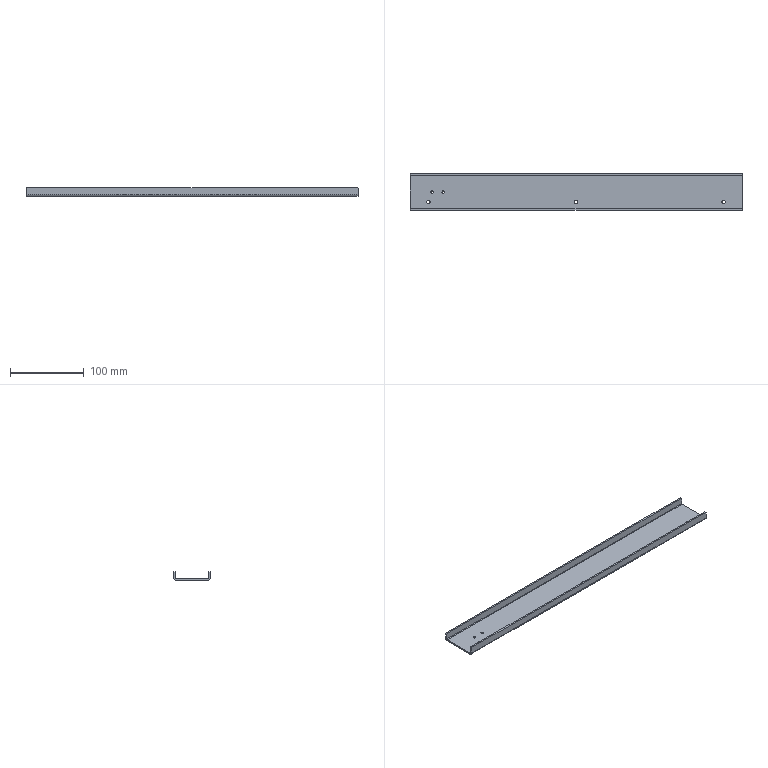Part | NX | features BREP 1 | 1 solid | 36 faces | box 450 x 49 x 12 mm | volume 60625 mm3 | plane 22 | cylinder 14 | commonest cylinder face diameters 4.5 x6 3.3 x4 1.473 x2 5.473 x2
STEP:
#1=CARTESIAN_POINT('',(27.25,9.,-2.));
#2=VERTEX_POINT('',#1);
#3=CARTESIAN_POINT('',(22.75,9.,-2.));
#4=VERTEX_POINT('',#3);
#5=CARTESIAN_POINT('',(25.,9.,-2.));
#6=DIRECTION('',(0.,0.,-1.));
#7=DIRECTION('',(-1.,0.,0.));
#8=AXIS2_PLACEMENT_3D('',#5,#6,#7);
#9=CIRCLE('',#8,2.25);
#10=EDGE_CURVE('',#2,#4,#9,.T.);
#11=ORIENTED_EDGE('',*,*,#10,.T.);
#12=CARTESIAN_POINT('',(22.75,9.,0.));
#13=VERTEX_POINT('',#12);
#14=CARTESIAN_POINT('',(22.75,9.,0.));
#15=DIRECTION('',(0.,0.,1.));
#16=VECTOR('',#15,1000.);
#17=LINE('',#14,#16);
#18=EDGE_CURVE('',#13,#4,#17,.F.);
#19=ORIENTED_EDGE('',*,*,#18,.F.);
#20=CARTESIAN_POINT('',(27.25,9.,0.));
#21=VERTEX_POINT('',#20);
#22=CARTESIAN_POINT('',(25.,9.,0.));
#23=DIRECTION('',(0.,0.,1.));
#24=DIRECTION('',(1.,0.,0.));
#25=AXIS2_PLACEMENT_3D('',#22,#23,#24);
#26=CIRCLE('',#25,2.25);
#27=EDGE_CURVE('',#13,#21,#26,.T.);
#28=ORIENTED_EDGE('',*,*,#27,.T.);
#29=CARTESIAN_POINT('',(27.25,9.,0.));
#30=DIRECTION('',(0.,0.,1.));
#31=VECTOR('',#30,1000.);
#32=LINE('',#29,#31);
#33=EDGE_CURVE('',#21,#2,#32,.F.);
#34=ORIENTED_EDGE('',*,*,#33,.T.);
#35=EDGE_LOOP('',(#11,#19,#28,#34));
#36=FACE_BOUND('',#35,.T.);
#37=CARTESIAN_POINT('',(25.,9.,0.));
#38=DIRECTION('',(0.,0.,1.));
#39=DIRECTION('',(1.,0.,0.));
#40=AXIS2_PLACEMENT_3D('',#37,#38,#39);
#41=CYLINDRICAL_SURFACE('',#40,2.25);
#42=ADVANCED_FACE('',(#36),#41,.F.);
#43=CARTESIAN_POINT('',(227.25,9.,-2.));
#44=VERTEX_POINT('',#43);
#45=CARTESIAN_POINT('',(222.75,9.,-2.));
#46=VERTEX_POINT('',#45);
#47=CARTESIAN_POINT('',(225.,9.,-2.));
#48=DIRECTION('',(0.,0.,-1.));
#49=DIRECTION('',(-1.,0.,0.));
#50=AXIS2_PLACEMENT_3D('',#47,#48,#49);
#51=CIRCLE('',#50,2.25);
#52=EDGE_CURVE('',#44,#46,#51,.T.);
#53=ORIENTED_EDGE('',*,*,#52,.T.);
#54=CARTESIAN_POINT('',(222.75,9.,0.));
#55=VERTEX_POINT('',#54);
#56=CARTESIAN_POINT('',(222.75,9.,0.));
#57=DIRECTION('',(0.,0.,1.));
#58=VECTOR('',#57,1000.);
#59=LINE('',#56,#58);
#60=EDGE_CURVE('',#55,#46,#59,.F.);
#61=ORIENTED_EDGE('',*,*,#60,.F.);
#62=CARTESIAN_POINT('',(227.25,9.,0.));
#63=VERTEX_POINT('',#62);
#64=CARTESIAN_POINT('',(225.,9.,0.));
#65=DIRECTION('',(0.,0.,1.));
#66=DIRECTION('',(1.,0.,0.));
#67=AXIS2_PLACEMENT_3D('',#64,#65,#66);
#68=CIRCLE('',#67,2.25);
#69=EDGE_CURVE('',#55,#63,#68,.T.);
#70=ORIENTED_EDGE('',*,*,#69,.T.);
#71=CARTESIAN_POINT('',(227.25,9.,0.));
#72=DIRECTION('',(0.,0.,1.));
#73=VECTOR('',#72,1000.);
#74=LINE('',#71,#73);
#75=EDGE_CURVE('',#63,#44,#74,.F.);
#76=ORIENTED_EDGE('',*,*,#75,.T.);
#77=EDGE_LOOP('',(#53,#61,#70,#76));
#78=FACE_BOUND('',#77,.T.);
#79=CARTESIAN_POINT('',(225.,9.,0.));
#80=DIRECTION('',(0.,0.,1.));
#81=DIRECTION('',(1.,0.,0.));
#82=AXIS2_PLACEMENT_3D('',#79,#80,#81);
#83=CYLINDRICAL_SURFACE('',#82,2.25);
#84=ADVANCED_FACE('',(#78),#83,.F.);
#85=CARTESIAN_POINT('',(427.25,9.,-2.));
#86=VERTEX_POINT('',#85);
#87=CARTESIAN_POINT('',(422.75,9.,-2.));
#88=VERTEX_POINT('',#87);
#89=CARTESIAN_POINT('',(425.,9.,-2.));
#90=DIRECTION('',(0.,0.,-1.));
#91=DIRECTION('',(-1.,0.,0.));
#92=AXIS2_PLACEMENT_3D('',#89,#90,#91);
#93=CIRCLE('',#92,2.25);
#94=EDGE_CURVE('',#86,#88,#93,.T.);
#95=ORIENTED_EDGE('',*,*,#94,.T.);
#96=CARTESIAN_POINT('',(422.75,9.,0.));
#97=VERTEX_POINT('',#96);
#98=CARTESIAN_POINT('',(422.75,9.,0.));
#99=DIRECTION('',(0.,0.,1.));
#100=VECTOR('',#99,1000.);
#101=LINE('',#98,#100);
#102=EDGE_CURVE('',#97,#88,#101,.F.);
#103=ORIENTED_EDGE('',*,*,#102,.F.);
#104=CARTESIAN_POINT('',(427.25,9.,0.));
#105=VERTEX_POINT('',#104);
#106=CARTESIAN_POINT('',(425.,9.,0.));
#107=DIRECTION('',(0.,0.,1.));
#108=DIRECTION('',(1.,0.,0.));
#109=AXIS2_PLACEMENT_3D('',#106,#107,#108);
#110=CIRCLE('',#109,2.25);
#111=EDGE_CURVE('',#97,#105,#110,.T.);
#112=ORIENTED_EDGE('',*,*,#111,.T.);
#113=CARTESIAN_POINT('',(427.25,9.,0.));
#114=DIRECTION('',(0.,0.,1.));
#115=VECTOR('',#114,1000.);
#116=LINE('',#113,#115);
#117=EDGE_CURVE('',#105,#86,#116,.F.);
#118=ORIENTED_EDGE('',*,*,#117,.T.);
#119=EDGE_LOOP('',(#95,#103,#112,#118));
#120=FACE_BOUND('',#119,.T.);
#121=CARTESIAN_POINT('',(425.,9.,0.));
#122=DIRECTION('',(0.,0.,1.));
#123=DIRECTION('',(1.,0.,0.));
#124=AXIS2_PLACEMENT_3D('',#121,#122,#123);
#125=CYLINDRICAL_SURFACE('',#124,2.25);
#126=ADVANCED_FACE('',(#120),#125,.F.);
#127=CARTESIAN_POINT('',(28.35,22.5,-2.));
#128=VERTEX_POINT('',#127);
#129=CARTESIAN_POINT('',(31.65,22.5,-2.));
#130=VERTEX_POINT('',#129);
#131=CARTESIAN_POINT('',(30.,22.5,-2.));
#132=DIRECTION('',(0.,0.,1.));
#133=DIRECTION('',(1.,0.,0.));
#134=AXIS2_PLACEMENT_3D('',#131,#132,#133);
#135=CIRCLE('',#134,1.65);
#136=EDGE_CURVE('',#128,#130,#135,.T.);
#137=ORIENTED_EDGE('',*,*,#136,.F.);
#138=CARTESIAN_POINT('',(28.35,22.5,0.));
#139=VERTEX_POINT('',#138);
#140=CARTESIAN_POINT('',(28.35,22.5,0.));
#141=DIRECTION('',(0.,0.,1.));
#142=VECTOR('',#141,1000.);
#143=LINE('',#140,#142);
#144=EDGE_CURVE('',#139,#128,#143,.F.);
#145=ORIENTED_EDGE('',*,*,#144,.F.);
#146=CARTESIAN_POINT('',(31.65,22.5,0.));
#147=VERTEX_POINT('',#146);
#148=CARTESIAN_POINT('',(30.,22.5,0.));
#149=DIRECTION('',(0.,0.,1.));
#150=DIRECTION('',(1.,0.,0.));
#151=AXIS2_PLACEMENT_3D('',#148,#149,#150);
#152=CIRCLE('',#151,1.65);
#153=EDGE_CURVE('',#139,#147,#152,.T.);
#154=ORIENTED_EDGE('',*,*,#153,.T.);
#155=CARTESIAN_POINT('',(31.65,22.5,0.));
#156=DIRECTION('',(0.,0.,1.));
#157=VECTOR('',#156,1000.);
#158=LINE('',#155,#157);
#159=EDGE_CURVE('',#147,#130,#158,.F.);
#160=ORIENTED_EDGE('',*,*,#159,.T.);
#161=EDGE_LOOP('',(#137,#145,#154,#160));
#162=FACE_BOUND('',#161,.T.);
#163=CARTESIAN_POINT('',(30.,22.5,0.));
#164=DIRECTION('',(0.,0.,1.));
#165=DIRECTION('',(1.,0.,0.));
#166=AXIS2_PLACEMENT_3D('',#163,#164,#165);
#167=CYLINDRICAL_SURFACE('',#166,1.65);
#168=ADVANCED_FACE('',(#162),#167,.F.);
#169=CARTESIAN_POINT('',(43.35,22.5,-2.));
#170=VERTEX_POINT('',#169);
#171=CARTESIAN_POINT('',(46.65,22.5,-2.));
#172=VERTEX_POINT('',#171);
#173=CARTESIAN_POINT('',(45.,22.5,-2.));
#174=DIRECTION('',(0.,0.,1.));
#175=DIRECTION('',(1.,0.,0.));
#176=AXIS2_PLACEMENT_3D('',#173,#174,#175);
#177=CIRCLE('',#176,1.65);
#178=EDGE_CURVE('',#170,#172,#177,.T.);
#179=ORIENTED_EDGE('',*,*,#178,.F.);
#180=CARTESIAN_POINT('',(43.35,22.5,0.));
#181=VERTEX_POINT('',#180);
#182=CARTESIAN_POINT('',(43.35,22.5,0.));
#183=DIRECTION('',(0.,0.,1.));
#184=VECTOR('',#183,1000.);
#185=LINE('',#182,#184);
#186=EDGE_CURVE('',#181,#170,#185,.F.);
#187=ORIENTED_EDGE('',*,*,#186,.F.);
#188=CARTESIAN_POINT('',(46.65,22.5,0.));
#189=VERTEX_POINT('',#188);
#190=CARTESIAN_POINT('',(45.,22.5,0.));
#191=DIRECTION('',(0.,0.,1.));
#192=DIRECTION('',(1.,0.,0.));
#193=AXIS2_PLACEMENT_3D('',#190,#191,#192);
#194=CIRCLE('',#193,1.65);
#195=EDGE_CURVE('',#181,#189,#194,.T.);
#196=ORIENTED_EDGE('',*,*,#195,.T.);
#197=CARTESIAN_POINT('',(46.65,22.5,0.));
#198=DIRECTION('',(0.,0.,1.));
#199=VECTOR('',#198,1000.);
#200=LINE('',#197,#199);
#201=EDGE_CURVE('',#189,#172,#200,.F.);
#202=ORIENTED_EDGE('',*,*,#201,.T.);
#203=EDGE_LOOP('',(#179,#187,#196,#202));
#204=FACE_BOUND('',#203,.T.);
#205=CARTESIAN_POINT('',(45.,22.5,0.));
#206=DIRECTION('',(0.,0.,1.));
#207=DIRECTION('',(1.,0.,0.));
#208=AXIS2_PLACEMENT_3D('',#205,#206,#207);
#209=CYLINDRICAL_SURFACE('',#208,1.65);
#210=ADVANCED_FACE('',(#204),#209,.F.);
#211=CARTESIAN_POINT('',(450.,0.7366,-2.));
#212=VERTEX_POINT('',#211);
#213=CARTESIAN_POINT('',(450.,44.263,-2.));
#214=VERTEX_POINT('',#213);
#215=CARTESIAN_POINT('',(450.,0.,-2.));
#216=DIRECTION('',(0.,1.,0.));
#217=VECTOR('',#216,1000.);
#218=LINE('',#215,#217);
#219=EDGE_CURVE('',#212,#214,#218,.T.);
#220=ORIENTED_EDGE('',*,*,#219,.F.);
#221=CARTESIAN_POINT('',(0.,0.7366,-2.));
#222=VERTEX_POINT('',#221);
#223=CARTESIAN_POINT('',(450.,0.7366,-2.));
#224=DIRECTION('',(-1.,0.,0.));
#225=VECTOR('',#224,1000.);
#226=LINE('',#223,#225);
#227=EDGE_CURVE('',#212,#222,#226,.T.);
#228=ORIENTED_EDGE('',*,*,#227,.T.);
#229=CARTESIAN_POINT('',(0.,44.263,-2.));
#230=VERTEX_POINT('',#229);
#231=CARTESIAN_POINT('',(0.,0.,-2.));
#232=DIRECTION('',(0.,-1.,0.));
#233=VECTOR('',#232,1000.);
#234=LINE('',#231,#233);
#235=EDGE_CURVE('',#230,#222,#234,.T.);
#236=ORIENTED_EDGE('',*,*,#235,.F.);
#237=CARTESIAN_POINT('',(0.,44.263,-2.));
#238=DIRECTION('',(1.,0.,0.));
#239=VECTOR('',#238,1000.);
#240=LINE('',#237,#239);
#241=EDGE_CURVE('',#230,#214,#240,.T.);
#242=ORIENTED_EDGE('',*,*,#241,.T.);
#243=EDGE_LOOP('',(#220,#228,#236,#242));
#244=FACE_BOUND('',#243,.T.);
#245=ORIENTED_EDGE('',*,*,#10,.F.);
#246=CARTESIAN_POINT('',(25.,9.,-2.));
#247=DIRECTION('',(0.,0.,-1.));
#248=DIRECTION('',(-1.,0.,0.));
#249=AXIS2_PLACEMENT_3D('',#246,#247,#248);
#250=CIRCLE('',#249,2.25);
#251=EDGE_CURVE('',#4,#2,#250,.T.);
#252=ORIENTED_EDGE('',*,*,#251,.F.);
#253=EDGE_LOOP('',(#245,#252));
#254=FACE_BOUND('',#253,.T.);
#255=ORIENTED_EDGE('',*,*,#52,.F.);
#256=CARTESIAN_POINT('',(225.,9.,-2.));
#257=DIRECTION('',(0.,0.,-1.));
#258=DIRECTION('',(-1.,0.,0.));
#259=AXIS2_PLACEMENT_3D('',#256,#257,#258);
#260=CIRCLE('',#259,2.25);
#261=EDGE_CURVE('',#46,#44,#260,.T.);
#262=ORIENTED_EDGE('',*,*,#261,.F.);
#263=EDGE_LOOP('',(#255,#262));
#264=FACE_BOUND('',#263,.T.);
#265=ORIENTED_EDGE('',*,*,#94,.F.);
#266=CARTESIAN_POINT('',(425.,9.,-2.));
#267=DIRECTION('',(0.,0.,-1.));
#268=DIRECTION('',(-1.,0.,0.));
#269=AXIS2_PLACEMENT_3D('',#266,#267,#268);
#270=CIRCLE('',#269,2.25);
#271=EDGE_CURVE('',#88,#86,#270,.T.);
#272=ORIENTED_EDGE('',*,*,#271,.F.);
#273=EDGE_LOOP('',(#265,#272));
#274=FACE_BOUND('',#273,.T.);
#275=CARTESIAN_POINT('',(30.,22.5,-2.));
#276=DIRECTION('',(0.,0.,1.));
#277=DIRECTION('',(1.,0.,0.));
#278=AXIS2_PLACEMENT_3D('',#275,#276,#277);
#279=CIRCLE('',#278,1.65);
#280=EDGE_CURVE('',#130,#128,#279,.T.);
#281=ORIENTED_EDGE('',*,*,#280,.T.);
#282=ORIENTED_EDGE('',*,*,#136,.T.);
#283=EDGE_LOOP('',(#281,#282));
#284=FACE_BOUND('',#283,.T.);
#285=CARTESIAN_POINT('',(45.,22.5,-2.));
#286=DIRECTION('',(0.,0.,1.));
#287=DIRECTION('',(1.,0.,0.));
#288=AXIS2_PLACEMENT_3D('',#285,#286,#287);
#289=CIRCLE('',#288,1.65);
#290=EDGE_CURVE('',#172,#170,#289,.T.);
#291=ORIENTED_EDGE('',*,*,#290,.T.);
#292=ORIENTED_EDGE('',*,*,#178,.T.);
#293=EDGE_LOOP('',(#291,#292));
#294=FACE_BOUND('',#293,.T.);
#295=CARTESIAN_POINT('',(0.,0.,-2.));
#296=DIRECTION('',(0.,0.,-1.));
#297=DIRECTION('',(0.,-1.,0.));
#298=AXIS2_PLACEMENT_3D('',#295,#296,#297);
#299=PLANE('',#298);
#300=ADVANCED_FACE('',(#244,#254,#264,#274,#284,#294),#299,.T.);
#301=CARTESIAN_POINT('',(450.,0.7366,0.));
#302=VERTEX_POINT('',#301);
#303=CARTESIAN_POINT('',(0.,0.7366,0.));
#304=VERTEX_POINT('',#303);
#305=CARTESIAN_POINT('',(450.,0.7366,0.));
#306=DIRECTION('',(-1.,0.,0.));
#307=VECTOR('',#306,1000.);
#308=LINE('',#305,#307);
#309=EDGE_CURVE('',#302,#304,#308,.T.);
#310=ORIENTED_EDGE('',*,*,#309,.F.);
#311=CARTESIAN_POINT('',(450.,44.263,0.));
#312=VERTEX_POINT('',#311);
#313=CARTESIAN_POINT('',(450.,0.,0.));
#314=DIRECTION('',(0.,1.,0.));
#315=VECTOR('',#314,1000.);
#316=LINE('',#313,#315);
#317=EDGE_CURVE('',#302,#312,#316,.T.);
#318=ORIENTED_EDGE('',*,*,#317,.T.);
#319=CARTESIAN_POINT('',(0.,44.263,0.));
#320=VERTEX_POINT('',#319);
#321=CARTESIAN_POINT('',(0.,44.263,0.));
#322=DIRECTION('',(1.,0.,0.));
#323=VECTOR('',#322,1000.);
#324=LINE('',#321,#323);
#325=EDGE_CURVE('',#320,#312,#324,.T.);
#326=ORIENTED_EDGE('',*,*,#325,.F.);
#327=CARTESIAN_POINT('',(0.,0.,0.));
#328=DIRECTION('',(0.,-1.,0.));
#329=VECTOR('',#328,1000.);
#330=LINE('',#327,#329);
#331=EDGE_CURVE('',#320,#304,#330,.T.);
#332=ORIENTED_EDGE('',*,*,#331,.T.);
#333=EDGE_LOOP('',(#310,#318,#326,#332));
#334=FACE_BOUND('',#333,.T.);
#335=CARTESIAN_POINT('',(25.,9.,0.));
#336=DIRECTION('',(0.,0.,1.));
#337=DIRECTION('',(1.,0.,0.));
#338=AXIS2_PLACEMENT_3D('',#335,#336,#337);
#339=CIRCLE('',#338,2.25);
#340=EDGE_CURVE('',#21,#13,#339,.T.);
#341=ORIENTED_EDGE('',*,*,#340,.F.);
#342=ORIENTED_EDGE('',*,*,#27,.F.);
#343=EDGE_LOOP('',(#341,#342));
#344=FACE_BOUND('',#343,.T.);
#345=CARTESIAN_POINT('',(225.,9.,0.));
#346=DIRECTION('',(0.,0.,1.));
#347=DIRECTION('',(1.,0.,0.));
#348=AXIS2_PLACEMENT_3D('',#345,#346,#347);
#349=CIRCLE('',#348,2.25);
#350=EDGE_CURVE('',#63,#55,#349,.T.);
#351=ORIENTED_EDGE('',*,*,#350,.F.);
#352=ORIENTED_EDGE('',*,*,#69,.F.);
#353=EDGE_LOOP('',(#351,#352));
#354=FACE_BOUND('',#353,.T.);
#355=CARTESIAN_POINT('',(425.,9.,0.));
#356=DIRECTION('',(0.,0.,1.));
#357=DIRECTION('',(1.,0.,0.));
#358=AXIS2_PLACEMENT_3D('',#355,#356,#357);
#359=CIRCLE('',#358,2.25);
#360=EDGE_CURVE('',#105,#97,#359,.T.);
#361=ORIENTED_EDGE('',*,*,#360,.F.);
#362=ORIENTED_EDGE('',*,*,#111,.F.);
#363=EDGE_LOOP('',(#361,#362));
#364=FACE_BOUND('',#363,.T.);
#365=CARTESIAN_POINT('',(30.,22.5,0.));
#366=DIRECTION('',(0.,0.,1.));
#367=DIRECTION('',(1.,0.,0.));
#368=AXIS2_PLACEMENT_3D('',#365,#366,#367);
#369=CIRCLE('',#368,1.65);
#370=EDGE_CURVE('',#147,#139,#369,.T.);
#371=ORIENTED_EDGE('',*,*,#370,.F.);
#372=ORIENTED_EDGE('',*,*,#153,.F.);
#373=EDGE_LOOP('',(#371,#372));
#374=FACE_BOUND('',#373,.T.);
#375=CARTESIAN_POINT('',(45.,22.5,0.));
#376=DIRECTION('',(0.,0.,1.));
#377=DIRECTION('',(1.,0.,0.));
#378=AXIS2_PLACEMENT_3D('',#375,#376,#377);
#379=CIRCLE('',#378,1.65);
#380=EDGE_CURVE('',#189,#181,#379,.T.);
#381=ORIENTED_EDGE('',*,*,#380,.F.);
#382=ORIENTED_EDGE('',*,*,#195,.F.);
#383=EDGE_LOOP('',(#381,#382));
#384=FACE_BOUND('',#383,.T.);
#385=CARTESIAN_POINT('',(0.,0.,0.));
#386=DIRECTION('',(0.,0.,-1.));
#387=DIRECTION('',(0.,-1.,0.));
#388=AXIS2_PLACEMENT_3D('',#385,#386,#387);
#389=PLANE('',#388);
#390=ADVANCED_FACE('',(#334,#344,#354,#364,#374,#384),#389,.F.);
#391=ORIENTED_EDGE('',*,*,#317,.F.);
#392=CARTESIAN_POINT('',(450.,0.7366,0.));
#393=DIRECTION('',(0.,0.,-1.));
#394=VECTOR('',#393,1000.);
#395=LINE('',#392,#394);
#396=EDGE_CURVE('',#302,#212,#395,.T.);
#397=ORIENTED_EDGE('',*,*,#396,.T.);
#398=ORIENTED_EDGE('',*,*,#219,.T.);
#399=CARTESIAN_POINT('',(450.,44.263,0.));
#400=DIRECTION('',(0.,0.,-1.));
#401=VECTOR('',#400,1000.);
#402=LINE('',#399,#401);
#403=EDGE_CURVE('',#312,#214,#402,.T.);
#404=ORIENTED_EDGE('',*,*,#403,.F.);
#405=EDGE_LOOP('',(#391,#397,#398,#404));
#406=FACE_BOUND('',#405,.T.);
#407=CARTESIAN_POINT('',(450.,0.,-2.));
#408=DIRECTION('',(1.,0.,0.));
#409=DIRECTION('',(0.,1.,0.));
#410=AXIS2_PLACEMENT_3D('',#407,#408,#409);
#411=PLANE('',#410);
#412=ADVANCED_FACE('',(#406),#411,.T.);
#413=CARTESIAN_POINT('',(0.,0.7366,0.));
#414=DIRECTION('',(0.,0.,-1.));
#415=VECTOR('',#414,1000.);
#416=LINE('',#413,#415);
#417=EDGE_CURVE('',#304,#222,#416,.T.);
#418=ORIENTED_EDGE('',*,*,#417,.F.);
#419=ORIENTED_EDGE('',*,*,#331,.F.);
#420=CARTESIAN_POINT('',(0.,44.263,0.));
#421=DIRECTION('',(0.,0.,-1.));
#422=VECTOR('',#421,1000.);
#423=LINE('',#420,#422);
#424=EDGE_CURVE('',#320,#230,#423,.T.);
#425=ORIENTED_EDGE('',*,*,#424,.T.);
#426=ORIENTED_EDGE('',*,*,#235,.T.);
#427=EDGE_LOOP('',(#418,#419,#425,#426));
#428=FACE_BOUND('',#427,.T.);
#429=CARTESIAN_POINT('',(0.,0.,-2.));
#430=DIRECTION('',(-1.,0.,0.));
#431=DIRECTION('',(0.,0.,1.));
#432=AXIS2_PLACEMENT_3D('',#429,#430,#431);
#433=PLANE('',#432);
#434=ADVANCED_FACE('',(#428),#433,.T.);
#435=CARTESIAN_POINT('',(450.,45.,0.7366));
#436=VERTEX_POINT('',#435);
#437=CARTESIAN_POINT('',(450.,47.,0.7366));
#438=VERTEX_POINT('',#437);
#439=CARTESIAN_POINT('',(450.,45.,0.7366));
#440=DIRECTION('',(0.,1.,0.));
#441=VECTOR('',#440,1000.);
#442=LINE('',#439,#441);
#443=EDGE_CURVE('',#436,#438,#442,.T.);
#444=ORIENTED_EDGE('',*,*,#443,.F.);
#445=CARTESIAN_POINT('',(450.,44.263,0.7366));
#446=DIRECTION('',(1.,0.,0.));
#447=DIRECTION('',(0.,0.,1.));
#448=AXIS2_PLACEMENT_3D('',#445,#446,#447);
#449=CIRCLE('',#448,0.7366);
#450=EDGE_CURVE('',#312,#436,#449,.T.);
#451=ORIENTED_EDGE('',*,*,#450,.F.);
#452=ORIENTED_EDGE('',*,*,#403,.T.);
#453=CARTESIAN_POINT('',(450.,44.263,0.7366));
#454=DIRECTION('',(1.,0.,0.));
#455=DIRECTION('',(0.,0.,1.));
#456=AXIS2_PLACEMENT_3D('',#453,#454,#455);
#457=CIRCLE('',#456,2.737);
#458=EDGE_CURVE('',#214,#438,#457,.T.);
#459=ORIENTED_EDGE('',*,*,#458,.T.);
#460=EDGE_LOOP('',(#444,#451,#452,#459));
#461=FACE_BOUND('',#460,.T.);
#462=CARTESIAN_POINT('',(450.,44.263,0.7366));
#463=DIRECTION('',(1.,0.,0.));
#464=DIRECTION('',(0.,1.,0.));
#465=AXIS2_PLACEMENT_3D('',#462,#463,#464);
#466=PLANE('',#465);
#467=ADVANCED_FACE('',(#461),#466,.T.);
#468=CARTESIAN_POINT('',(0.,45.,0.7366));
#469=VERTEX_POINT('',#468);
#470=CARTESIAN_POINT('',(0.,44.263,0.7366));
#471=DIRECTION('',(-1.,0.,0.));
#472=DIRECTION('',(0.,0.,1.));
#473=AXIS2_PLACEMENT_3D('',#470,#471,#472);
#474=CIRCLE('',#473,0.7366);
#475=EDGE_CURVE('',#469,#320,#474,.T.);
#476=ORIENTED_EDGE('',*,*,#475,.F.);
#477=CARTESIAN_POINT('',(0.,47.,0.7366));
#478=VERTEX_POINT('',#477);
#479=CARTESIAN_POINT('',(0.,45.,0.7366));
#480=DIRECTION('',(0.,1.,0.));
#481=VECTOR('',#480,1000.);
#482=LINE('',#479,#481);
#483=EDGE_CURVE('',#469,#478,#482,.T.);
#484=ORIENTED_EDGE('',*,*,#483,.T.);
#485=CARTESIAN_POINT('',(0.,44.263,0.7366));
#486=DIRECTION('',(-1.,0.,0.));
#487=DIRECTION('',(0.,0.,1.));
#488=AXIS2_PLACEMENT_3D('',#485,#486,#487);
#489=CIRCLE('',#488,2.737);
#490=EDGE_CURVE('',#478,#230,#489,.T.);
#491=ORIENTED_EDGE('',*,*,#490,.T.);
#492=ORIENTED_EDGE('',*,*,#424,.F.);
#493=EDGE_LOOP('',(#476,#484,#491,#492));
#494=FACE_BOUND('',#493,.T.);
#495=CARTESIAN_POINT('',(0.,44.263,0.7366));
#496=DIRECTION('',(1.,0.,0.));
#497=DIRECTION('',(0.,1.,0.));
#498=AXIS2_PLACEMENT_3D('',#495,#496,#497);
#499=PLANE('',#498);
#500=ADVANCED_FACE('',(#494),#499,.F.);
#501=ORIENTED_EDGE('',*,*,#241,.F.);
#502=ORIENTED_EDGE('',*,*,#490,.F.);
#503=CARTESIAN_POINT('',(0.,47.,0.7366));
#504=DIRECTION('',(1.,0.,0.));
#505=VECTOR('',#504,1000.);
#506=LINE('',#503,#505);
#507=EDGE_CURVE('',#478,#438,#506,.T.);
#508=ORIENTED_EDGE('',*,*,#507,.T.);
#509=ORIENTED_EDGE('',*,*,#458,.F.);
#510=EDGE_LOOP('',(#501,#502,#508,#509));
#511=FACE_BOUND('',#510,.T.);
#512=CARTESIAN_POINT('',(0.,44.263,0.7366));
#513=DIRECTION('',(-1.,0.,0.));
#514=DIRECTION('',(0.,1.,0.));
#515=AXIS2_PLACEMENT_3D('',#512,#513,#514);
#516=CYLINDRICAL_SURFACE('',#515,2.737);
#517=ADVANCED_FACE('',(#511),#516,.T.);
#518=ORIENTED_EDGE('',*,*,#325,.T.);
#519=ORIENTED_EDGE('',*,*,#450,.T.);
#520=CARTESIAN_POINT('',(450.,45.,0.7366));
#521=DIRECTION('',(-1.,0.,0.));
#522=VECTOR('',#521,1000.);
#523=LINE('',#520,#522);
#524=EDGE_CURVE('',#436,#469,#523,.T.);
#525=ORIENTED_EDGE('',*,*,#524,.T.);
#526=ORIENTED_EDGE('',*,*,#475,.T.);
#527=EDGE_LOOP('',(#518,#519,#525,#526));
#528=FACE_BOUND('',#527,.T.);
#529=CARTESIAN_POINT('',(0.,44.263,0.7366));
#530=DIRECTION('',(-1.,0.,0.));
#531=DIRECTION('',(0.,1.,0.));
#532=AXIS2_PLACEMENT_3D('',#529,#530,#531);
#533=CYLINDRICAL_SURFACE('',#532,0.7366);
#534=ADVANCED_FACE('',(#528),#533,.F.);
#535=CARTESIAN_POINT('',(450.,47.,9.));
#536=VERTEX_POINT('',#535);
#537=CARTESIAN_POINT('',(450.,47.,0.));
#538=DIRECTION('',(0.,0.,-1.));
#539=VECTOR('',#538,1000.);
#540=LINE('',#537,#539);
#541=EDGE_CURVE('',#536,#438,#540,.T.);
#542=ORIENTED_EDGE('',*,*,#541,.F.);
#543=CARTESIAN_POINT('',(450.,45.,9.));
#544=VERTEX_POINT('',#543);
#545=CARTESIAN_POINT('',(450.,47.,9.));
#546=DIRECTION('',(0.,-1.,0.));
#547=VECTOR('',#546,1000.);
#548=LINE('',#545,#547);
#549=EDGE_CURVE('',#536,#544,#548,.T.);
#550=ORIENTED_EDGE('',*,*,#549,.T.);
#551=CARTESIAN_POINT('',(450.,45.,0.));
#552=DIRECTION('',(0.,0.,-1.));
#553=VECTOR('',#552,1000.);
#554=LINE('',#551,#553);
#555=EDGE_CURVE('',#544,#436,#554,.T.);
#556=ORIENTED_EDGE('',*,*,#555,.T.);
#557=ORIENTED_EDGE('',*,*,#443,.T.);
#558=EDGE_LOOP('',(#542,#550,#556,#557));
#559=FACE_BOUND('',#558,.T.);
#560=CARTESIAN_POINT('',(450.,47.,0.));
#561=DIRECTION('',(-1.,0.,0.));
#562=DIRECTION('',(0.,0.,1.));
#563=AXIS2_PLACEMENT_3D('',#560,#561,#562);
#564=PLANE('',#563);
#565=ADVANCED_FACE('',(#559),#564,.F.);
#566=CARTESIAN_POINT('',(0.,45.,9.));
#567=VERTEX_POINT('',#566);
#568=CARTESIAN_POINT('',(0.,45.,10.));
#569=DIRECTION('',(0.,0.,1.));
#570=VECTOR('',#569,1000.);
#571=LINE('',#568,#570);
#572=EDGE_CURVE('',#469,#567,#571,.T.);
#573=ORIENTED_EDGE('',*,*,#572,.T.);
#574=CARTESIAN_POINT('',(0.,47.,9.));
#575=VERTEX_POINT('',#574);
#576=CARTESIAN_POINT('',(0.,47.,9.));
#577=DIRECTION('',(0.,1.,0.));
#578=VECTOR('',#577,1000.);
#579=LINE('',#576,#578);
#580=EDGE_CURVE('',#567,#575,#579,.T.);
#581=ORIENTED_EDGE('',*,*,#580,.T.);
#582=CARTESIAN_POINT('',(0.,47.,10.));
#583=DIRECTION('',(0.,0.,1.));
#584=VECTOR('',#583,1000.);
#585=LINE('',#582,#584);
#586=EDGE_CURVE('',#478,#575,#585,.T.);
#587=ORIENTED_EDGE('',*,*,#586,.F.);
#588=ORIENTED_EDGE('',*,*,#483,.F.);
#589=EDGE_LOOP('',(#573,#581,#587,#588));
#590=FACE_BOUND('',#589,.T.);
#591=CARTESIAN_POINT('',(0.,47.,10.));
#592=DIRECTION('',(1.,0.,0.));
#593=DIRECTION('',(0.,1.,0.));
#594=AXIS2_PLACEMENT_3D('',#591,#592,#593);
#595=PLANE('',#594);
#596=ADVANCED_FACE('',(#590),#595,.F.);
#597=CARTESIAN_POINT('',(1.,47.,10.));
#598=VERTEX_POINT('',#597);
#599=CARTESIAN_POINT('',(449.,47.,10.));
#600=VERTEX_POINT('',#599);
#601=CARTESIAN_POINT('',(450.,47.,10.));
#602=DIRECTION('',(1.,0.,0.));
#603=VECTOR('',#602,1000.);
#604=LINE('',#601,#603);
#605=EDGE_CURVE('',#598,#600,#604,.T.);
#606=ORIENTED_EDGE('',*,*,#605,.T.);
#607=CARTESIAN_POINT('',(450.,47.,9.));
#608=DIRECTION('',(0.7071,0.,-0.7071));
#609=VECTOR('',#608,1000.);
#610=LINE('',#607,#609);
#611=EDGE_CURVE('',#600,#536,#610,.T.);
#612=ORIENTED_EDGE('',*,*,#611,.T.);
#613=ORIENTED_EDGE('',*,*,#541,.T.);
#614=ORIENTED_EDGE('',*,*,#507,.F.);
#615=ORIENTED_EDGE('',*,*,#586,.T.);
#616=CARTESIAN_POINT('',(1.,47.,10.));
#617=DIRECTION('',(0.7071,0.,0.7071));
#618=VECTOR('',#617,1000.);
#619=LINE('',#616,#618);
#620=EDGE_CURVE('',#575,#598,#619,.T.);
#621=ORIENTED_EDGE('',*,*,#620,.T.);
#622=EDGE_LOOP('',(#606,#612,#613,#614,#615,#621));
#623=FACE_BOUND('',#622,.T.);
#624=CARTESIAN_POINT('',(0.,47.,0.));
#625=DIRECTION('',(0.,-1.,0.));
#626=DIRECTION('',(-1.,0.,0.));
#627=AXIS2_PLACEMENT_3D('',#624,#625,#626);
#628=PLANE('',#627);
#629=ADVANCED_FACE('',(#623),#628,.F.);
#630=ORIENTED_EDGE('',*,*,#555,.F.);
#631=CARTESIAN_POINT('',(449.,45.,10.));
#632=VERTEX_POINT('',#631);
#633=CARTESIAN_POINT('',(229.5,45.,229.5));
#634=DIRECTION('',(-0.7071,0.,0.7071));
#635=VECTOR('',#634,1000.);
#636=LINE('',#633,#635);
#637=EDGE_CURVE('',#544,#632,#636,.T.);
#638=ORIENTED_EDGE('',*,*,#637,.T.);
#639=CARTESIAN_POINT('',(1.,45.,10.));
#640=VERTEX_POINT('',#639);
#641=CARTESIAN_POINT('',(450.,45.,10.));
#642=DIRECTION('',(1.,0.,0.));
#643=VECTOR('',#642,1000.);
#644=LINE('',#641,#643);
#645=EDGE_CURVE('',#640,#632,#644,.T.);
#646=ORIENTED_EDGE('',*,*,#645,.F.);
#647=CARTESIAN_POINT('',(-4.5,45.,4.5));
#648=DIRECTION('',(-0.7071,0.,-0.7071));
#649=VECTOR('',#648,1000.);
#650=LINE('',#647,#649);
#651=EDGE_CURVE('',#640,#567,#650,.T.);
#652=ORIENTED_EDGE('',*,*,#651,.T.);
#653=ORIENTED_EDGE('',*,*,#572,.F.);
#654=ORIENTED_EDGE('',*,*,#524,.F.);
#655=EDGE_LOOP('',(#630,#638,#646,#652,#653,#654));
#656=FACE_BOUND('',#655,.T.);
#657=CARTESIAN_POINT('',(0.,45.,0.));
#658=DIRECTION('',(0.,-1.,0.));
#659=DIRECTION('',(-1.,0.,0.));
#660=AXIS2_PLACEMENT_3D('',#657,#658,#659);
#661=PLANE('',#660);
#662=ADVANCED_FACE('',(#656),#661,.T.);
#663=ORIENTED_EDGE('',*,*,#645,.T.);
#664=CARTESIAN_POINT('',(449.,47.,10.));
#665=DIRECTION('',(0.,1.,0.));
#666=VECTOR('',#665,1000.);
#667=LINE('',#664,#666);
#668=EDGE_CURVE('',#632,#600,#667,.T.);
#669=ORIENTED_EDGE('',*,*,#668,.T.);
#670=ORIENTED_EDGE('',*,*,#605,.F.);
#671=CARTESIAN_POINT('',(1.,47.,10.));
#672=DIRECTION('',(0.,-1.,0.));
#673=VECTOR('',#672,1000.);
#674=LINE('',#671,#673);
#675=EDGE_CURVE('',#598,#640,#674,.T.);
#676=ORIENTED_EDGE('',*,*,#675,.T.);
#677=EDGE_LOOP('',(#663,#669,#670,#676));
#678=FACE_BOUND('',#677,.T.);
#679=CARTESIAN_POINT('',(450.,47.,10.));
#680=DIRECTION('',(0.,0.,-1.));
#681=DIRECTION('',(0.,-1.,0.));
#682=AXIS2_PLACEMENT_3D('',#679,#680,#681);
#683=PLANE('',#682);
#684=ADVANCED_FACE('',(#678),#683,.F.);
#685=CARTESIAN_POINT('',(0.,0.,0.7366));
#686=VERTEX_POINT('',#685);
#687=CARTESIAN_POINT('',(0.,-2.,0.7366));
#688=VERTEX_POINT('',#687);
#689=CARTESIAN_POINT('',(0.,0.,0.7366));
#690=DIRECTION('',(0.,-1.,0.));
#691=VECTOR('',#690,1000.);
#692=LINE('',#689,#691);
#693=EDGE_CURVE('',#686,#688,#692,.T.);
#694=ORIENTED_EDGE('',*,*,#693,.F.);
#695=CARTESIAN_POINT('',(0.,0.7366,0.7366));
#696=DIRECTION('',(-1.,0.,0.));
#697=DIRECTION('',(0.,1.,0.));
#698=AXIS2_PLACEMENT_3D('',#695,#696,#697);
#699=CIRCLE('',#698,0.7366);
#700=EDGE_CURVE('',#304,#686,#699,.T.);
#701=ORIENTED_EDGE('',*,*,#700,.F.);
#702=ORIENTED_EDGE('',*,*,#417,.T.);
#703=CARTESIAN_POINT('',(0.,0.7366,0.7366));
#704=DIRECTION('',(-1.,0.,0.));
#705=DIRECTION('',(0.,1.,0.));
#706=AXIS2_PLACEMENT_3D('',#703,#704,#705);
#707=CIRCLE('',#706,2.737);
#708=EDGE_CURVE('',#222,#688,#707,.T.);
#709=ORIENTED_EDGE('',*,*,#708,.T.);
#710=EDGE_LOOP('',(#694,#701,#702,#709));
#711=FACE_BOUND('',#710,.T.);
#712=CARTESIAN_POINT('',(0.,0.7366,0.7366));
#713=DIRECTION('',(-1.,0.,0.));
#714=DIRECTION('',(0.,1.,0.));
#715=AXIS2_PLACEMENT_3D('',#712,#713,#714);
#716=PLANE('',#715);
#717=ADVANCED_FACE('',(#711),#716,.T.);
#718=CARTESIAN_POINT('',(450.,0.,0.7366));
#719=VERTEX_POINT('',#718);
#720=CARTESIAN_POINT('',(450.,0.7366,0.7366));
#721=DIRECTION('',(1.,0.,0.));
#722=DIRECTION('',(0.,1.,0.));
#723=AXIS2_PLACEMENT_3D('',#720,#721,#722);
#724=CIRCLE('',#723,0.7366);
#725=EDGE_CURVE('',#719,#302,#724,.T.);
#726=ORIENTED_EDGE('',*,*,#725,.F.);
#727=CARTESIAN_POINT('',(450.,-2.,0.7366));
#728=VERTEX_POINT('',#727);
#729=CARTESIAN_POINT('',(450.,0.,0.7366));
#730=DIRECTION('',(0.,-1.,0.));
#731=VECTOR('',#730,1000.);
#732=LINE('',#729,#731);
#733=EDGE_CURVE('',#719,#728,#732,.T.);
#734=ORIENTED_EDGE('',*,*,#733,.T.);
#735=CARTESIAN_POINT('',(450.,0.7366,0.7366));
#736=DIRECTION('',(1.,0.,0.));
#737=DIRECTION('',(0.,1.,0.));
#738=AXIS2_PLACEMENT_3D('',#735,#736,#737);
#739=CIRCLE('',#738,2.737);
#740=EDGE_CURVE('',#728,#212,#739,.T.);
#741=ORIENTED_EDGE('',*,*,#740,.T.);
#742=ORIENTED_EDGE('',*,*,#396,.F.);
#743=EDGE_LOOP('',(#726,#734,#741,#742));
#744=FACE_BOUND('',#743,.T.);
#745=CARTESIAN_POINT('',(450.,0.7366,0.7366));
#746=DIRECTION('',(-1.,0.,0.));
#747=DIRECTION('',(0.,1.,0.));
#748=AXIS2_PLACEMENT_3D('',#745,#746,#747);
#749=PLANE('',#748);
#750=ADVANCED_FACE('',(#744),#749,.F.);
#751=ORIENTED_EDGE('',*,*,#227,.F.);
#752=ORIENTED_EDGE('',*,*,#740,.F.);
#753=CARTESIAN_POINT('',(0.,-2.,0.7366));
#754=DIRECTION('',(-1.,0.,0.));
#755=VECTOR('',#754,1000.);
#756=LINE('',#753,#755);
#757=EDGE_CURVE('',#728,#688,#756,.T.);
#758=ORIENTED_EDGE('',*,*,#757,.T.);
#759=ORIENTED_EDGE('',*,*,#708,.F.);
#760=EDGE_LOOP('',(#751,#752,#758,#759));
#761=FACE_BOUND('',#760,.T.);
#762=CARTESIAN_POINT('',(450.,0.7366,0.7366));
#763=DIRECTION('',(1.,0.,0.));
#764=DIRECTION('',(0.,-1.,0.));
#765=AXIS2_PLACEMENT_3D('',#762,#763,#764);
#766=CYLINDRICAL_SURFACE('',#765,2.737);
#767=ADVANCED_FACE('',(#761),#766,.T.);
#768=ORIENTED_EDGE('',*,*,#309,.T.);
#769=ORIENTED_EDGE('',*,*,#700,.T.);
#770=CARTESIAN_POINT('',(0.,0.,0.7366));
#771=DIRECTION('',(1.,0.,0.));
#772=VECTOR('',#771,1000.);
#773=LINE('',#770,#772);
#774=EDGE_CURVE('',#686,#719,#773,.T.);
#775=ORIENTED_EDGE('',*,*,#774,.T.);
#776=ORIENTED_EDGE('',*,*,#725,.T.);
#777=EDGE_LOOP('',(#768,#769,#775,#776));
#778=FACE_BOUND('',#777,.T.);
#779=CARTESIAN_POINT('',(450.,0.7366,0.7366));
#780=DIRECTION('',(1.,0.,0.));
#781=DIRECTION('',(0.,-1.,0.));
#782=AXIS2_PLACEMENT_3D('',#779,#780,#781);
#783=CYLINDRICAL_SURFACE('',#782,0.7366);
#784=ADVANCED_FACE('',(#778),#783,.F.);
#785=CARTESIAN_POINT('',(0.,-2.,9.));
#786=VERTEX_POINT('',#785);
#787=CARTESIAN_POINT('',(0.,-2.,0.));
#788=DIRECTION('',(0.,0.,-1.));
#789=VECTOR('',#788,1000.);
#790=LINE('',#787,#789);
#791=EDGE_CURVE('',#786,#688,#790,.T.);
#792=ORIENTED_EDGE('',*,*,#791,.F.);
#793=CARTESIAN_POINT('',(0.,0.,9.));
#794=VERTEX_POINT('',#793);
#795=CARTESIAN_POINT('',(0.,-2.,9.));
#796=DIRECTION('',(0.,1.,0.));
#797=VECTOR('',#796,1000.);
#798=LINE('',#795,#797);
#799=EDGE_CURVE('',#786,#794,#798,.T.);
#800=ORIENTED_EDGE('',*,*,#799,.T.);
#801=CARTESIAN_POINT('',(0.,0.,0.));
#802=DIRECTION('',(0.,0.,-1.));
#803=VECTOR('',#802,1000.);
#804=LINE('',#801,#803);
#805=EDGE_CURVE('',#794,#686,#804,.T.);
#806=ORIENTED_EDGE('',*,*,#805,.T.);
#807=ORIENTED_EDGE('',*,*,#693,.T.);
#808=EDGE_LOOP('',(#792,#800,#806,#807));
#809=FACE_BOUND('',#808,.T.);
#810=CARTESIAN_POINT('',(0.,-2.,0.));
#811=DIRECTION('',(1.,0.,0.));
#812=DIRECTION('',(0.,1.,0.));
#813=AXIS2_PLACEMENT_3D('',#810,#811,#812);
#814=PLANE('',#813);
#815=ADVANCED_FACE('',(#809),#814,.F.);
#816=CARTESIAN_POINT('',(450.,0.,9.));
#817=VERTEX_POINT('',#816);
#818=CARTESIAN_POINT('',(450.,0.,10.));
#819=DIRECTION('',(0.,0.,1.));
#820=VECTOR('',#819,1000.);
#821=LINE('',#818,#820);
#822=EDGE_CURVE('',#719,#817,#821,.T.);
#823=ORIENTED_EDGE('',*,*,#822,.T.);
#824=CARTESIAN_POINT('',(450.,-2.,9.));
#825=VERTEX_POINT('',#824);
#826=CARTESIAN_POINT('',(450.,-2.,9.));
#827=DIRECTION('',(0.,-1.,0.));
#828=VECTOR('',#827,1000.);
#829=LINE('',#826,#828);
#830=EDGE_CURVE('',#817,#825,#829,.T.);
#831=ORIENTED_EDGE('',*,*,#830,.T.);
#832=CARTESIAN_POINT('',(450.,-2.,10.));
#833=DIRECTION('',(0.,0.,1.));
#834=VECTOR('',#833,1000.);
#835=LINE('',#832,#834);
#836=EDGE_CURVE('',#728,#825,#835,.T.);
#837=ORIENTED_EDGE('',*,*,#836,.F.);
#838=ORIENTED_EDGE('',*,*,#733,.F.);
#839=EDGE_LOOP('',(#823,#831,#837,#838));
#840=FACE_BOUND('',#839,.T.);
#841=CARTESIAN_POINT('',(450.,-2.,10.));
#842=DIRECTION('',(-1.,0.,0.));
#843=DIRECTION('',(0.,0.,1.));
#844=AXIS2_PLACEMENT_3D('',#841,#842,#843);
#845=PLANE('',#844);
#846=ADVANCED_FACE('',(#840),#845,.F.);
#847=ORIENTED_EDGE('',*,*,#836,.T.);
#848=CARTESIAN_POINT('',(449.,-2.,10.));
#849=VERTEX_POINT('',#848);
#850=CARTESIAN_POINT('',(449.,-2.,10.));
#851=DIRECTION('',(-0.7071,0.,0.7071));
#852=VECTOR('',#851,1000.);
#853=LINE('',#850,#852);
#854=EDGE_CURVE('',#825,#849,#853,.T.);
#855=ORIENTED_EDGE('',*,*,#854,.T.);
#856=CARTESIAN_POINT('',(1.,-2.,10.));
#857=VERTEX_POINT('',#856);
#858=CARTESIAN_POINT('',(0.,-2.,10.));
#859=DIRECTION('',(-1.,0.,0.));
#860=VECTOR('',#859,1000.);
#861=LINE('',#858,#860);
#862=EDGE_CURVE('',#849,#857,#861,.T.);
#863=ORIENTED_EDGE('',*,*,#862,.T.);
#864=CARTESIAN_POINT('',(0.,-2.,9.));
#865=DIRECTION('',(-0.7071,0.,-0.7071));
#866=VECTOR('',#865,1000.);
#867=LINE('',#864,#866);
#868=EDGE_CURVE('',#857,#786,#867,.T.);
#869=ORIENTED_EDGE('',*,*,#868,.T.);
#870=ORIENTED_EDGE('',*,*,#791,.T.);
#871=ORIENTED_EDGE('',*,*,#757,.F.);
#872=EDGE_LOOP('',(#847,#855,#863,#869,#870,#871));
#873=FACE_BOUND('',#872,.T.);
#874=CARTESIAN_POINT('',(0.,-2.,0.));
#875=DIRECTION('',(0.,1.,0.));
#876=DIRECTION('',(0.,0.,-1.));
#877=AXIS2_PLACEMENT_3D('',#874,#875,#876);
#878=PLANE('',#877);
#879=ADVANCED_FACE('',(#873),#878,.F.);
#880=CARTESIAN_POINT('',(449.,0.,10.));
#881=VERTEX_POINT('',#880);
#882=CARTESIAN_POINT('',(1.,0.,10.));
#883=VERTEX_POINT('',#882);
#884=CARTESIAN_POINT('',(0.,0.,10.));
#885=DIRECTION('',(-1.,0.,0.));
#886=VECTOR('',#885,1000.);
#887=LINE('',#884,#886);
#888=EDGE_CURVE('',#881,#883,#887,.T.);
#889=ORIENTED_EDGE('',*,*,#888,.F.);
#890=CARTESIAN_POINT('',(229.5,0.,229.5));
#891=DIRECTION('',(0.7071,0.,-0.7071));
#892=VECTOR('',#891,1000.);
#893=LINE('',#890,#892);
#894=EDGE_CURVE('',#881,#817,#893,.T.);
#895=ORIENTED_EDGE('',*,*,#894,.T.);
#896=ORIENTED_EDGE('',*,*,#822,.F.);
#897=ORIENTED_EDGE('',*,*,#774,.F.);
#898=ORIENTED_EDGE('',*,*,#805,.F.);
#899=CARTESIAN_POINT('',(-4.5,0.,4.5));
#900=DIRECTION('',(0.7071,0.,0.7071));
#901=VECTOR('',#900,1000.);
#902=LINE('',#899,#901);
#903=EDGE_CURVE('',#794,#883,#902,.T.);
#904=ORIENTED_EDGE('',*,*,#903,.T.);
#905=EDGE_LOOP('',(#889,#895,#896,#897,#898,#904));
#906=FACE_BOUND('',#905,.T.);
#907=CARTESIAN_POINT('',(0.,0.,0.));
#908=DIRECTION('',(0.,1.,0.));
#909=DIRECTION('',(0.,0.,-1.));
#910=AXIS2_PLACEMENT_3D('',#907,#908,#909);
#911=PLANE('',#910);
#912=ADVANCED_FACE('',(#906),#911,.T.);
#913=ORIENTED_EDGE('',*,*,#862,.F.);
#914=CARTESIAN_POINT('',(449.,-2.,10.));
#915=DIRECTION('',(0.,1.,0.));
#916=VECTOR('',#915,1000.);
#917=LINE('',#914,#916);
#918=EDGE_CURVE('',#849,#881,#917,.T.);
#919=ORIENTED_EDGE('',*,*,#918,.T.);
#920=ORIENTED_EDGE('',*,*,#888,.T.);
#921=CARTESIAN_POINT('',(1.,-2.,10.));
#922=DIRECTION('',(0.,-1.,0.));
#923=VECTOR('',#922,1000.);
#924=LINE('',#921,#923);
#925=EDGE_CURVE('',#883,#857,#924,.T.);
#926=ORIENTED_EDGE('',*,*,#925,.T.);
#927=EDGE_LOOP('',(#913,#919,#920,#926));
#928=FACE_BOUND('',#927,.T.);
#929=CARTESIAN_POINT('',(0.,-2.,10.));
#930=DIRECTION('',(0.,0.,-1.));
#931=DIRECTION('',(-1.,0.,0.));
#932=AXIS2_PLACEMENT_3D('',#929,#930,#931);
#933=PLANE('',#932);
#934=ADVANCED_FACE('',(#928),#933,.F.);
#935=ORIENTED_EDGE('',*,*,#186,.T.);
#936=ORIENTED_EDGE('',*,*,#290,.F.);
#937=ORIENTED_EDGE('',*,*,#201,.F.);
#938=ORIENTED_EDGE('',*,*,#380,.T.);
#939=EDGE_LOOP('',(#935,#936,#937,#938));
#940=FACE_BOUND('',#939,.T.);
#941=CARTESIAN_POINT('',(45.,22.5,0.));
#942=DIRECTION('',(0.,0.,1.));
#943=DIRECTION('',(1.,0.,0.));
#944=AXIS2_PLACEMENT_3D('',#941,#942,#943);
#945=CYLINDRICAL_SURFACE('',#944,1.65);
#946=ADVANCED_FACE('',(#940),#945,.F.);
#947=ORIENTED_EDGE('',*,*,#144,.T.);
#948=ORIENTED_EDGE('',*,*,#280,.F.);
#949=ORIENTED_EDGE('',*,*,#159,.F.);
#950=ORIENTED_EDGE('',*,*,#370,.T.);
#951=EDGE_LOOP('',(#947,#948,#949,#950));
#952=FACE_BOUND('',#951,.T.);
#953=CARTESIAN_POINT('',(30.,22.5,0.));
#954=DIRECTION('',(0.,0.,1.));
#955=DIRECTION('',(1.,0.,0.));
#956=AXIS2_PLACEMENT_3D('',#953,#954,#955);
#957=CYLINDRICAL_SURFACE('',#956,1.65);
#958=ADVANCED_FACE('',(#952),#957,.F.);
#959=ORIENTED_EDGE('',*,*,#611,.F.);
#960=ORIENTED_EDGE('',*,*,#668,.F.);
#961=ORIENTED_EDGE('',*,*,#637,.F.);
#962=ORIENTED_EDGE('',*,*,#549,.F.);
#963=EDGE_LOOP('',(#959,#960,#961,#962));
#964=FACE_BOUND('',#963,.T.);
#965=CARTESIAN_POINT('',(450.,47.,9.));
#966=DIRECTION('',(-0.7071,0.,-0.7071));
#967=DIRECTION('',(-0.7071,0.,0.7071));
#968=AXIS2_PLACEMENT_3D('',#965,#966,#967);
#969=PLANE('',#968);
#970=ADVANCED_FACE('',(#964),#969,.F.);
#971=ORIENTED_EDGE('',*,*,#854,.F.);
#972=ORIENTED_EDGE('',*,*,#830,.F.);
#973=ORIENTED_EDGE('',*,*,#894,.F.);
#974=ORIENTED_EDGE('',*,*,#918,.F.);
#975=EDGE_LOOP('',(#971,#972,#973,#974));
#976=FACE_BOUND('',#975,.T.);
#977=CARTESIAN_POINT('',(449.,-2.,10.));
#978=DIRECTION('',(-0.7071,0.,-0.7071));
#979=DIRECTION('',(-0.7071,0.,0.7071));
#980=AXIS2_PLACEMENT_3D('',#977,#978,#979);
#981=PLANE('',#980);
#982=ADVANCED_FACE('',(#976),#981,.F.);
#983=ORIENTED_EDGE('',*,*,#620,.F.);
#984=ORIENTED_EDGE('',*,*,#580,.F.);
#985=ORIENTED_EDGE('',*,*,#651,.F.);
#986=ORIENTED_EDGE('',*,*,#675,.F.);
#987=EDGE_LOOP('',(#983,#984,#985,#986));
#988=FACE_BOUND('',#987,.T.);
#989=CARTESIAN_POINT('',(1.,47.,10.));
#990=DIRECTION('',(0.7071,0.,-0.7071));
#991=DIRECTION('',(0.,-1.,0.));
#992=AXIS2_PLACEMENT_3D('',#989,#990,#991);
#993=PLANE('',#992);
#994=ADVANCED_FACE('',(#988),#993,.F.);
#995=ORIENTED_EDGE('',*,*,#868,.F.);
#996=ORIENTED_EDGE('',*,*,#925,.F.);
#997=ORIENTED_EDGE('',*,*,#903,.F.);
#998=ORIENTED_EDGE('',*,*,#799,.F.);
#999=EDGE_LOOP('',(#995,#996,#997,#998));
#1000=FACE_BOUND('',#999,.T.);
#1001=CARTESIAN_POINT('',(0.,-2.,9.));
#1002=DIRECTION('',(0.7071,0.,-0.7071));
#1003=DIRECTION('',(0.,-1.,0.));
#1004=AXIS2_PLACEMENT_3D('',#1001,#1002,#1003);
#1005=PLANE('',#1004);
#1006=ADVANCED_FACE('',(#1000),#1005,.F.);
#1007=ORIENTED_EDGE('',*,*,#102,.T.);
#1008=ORIENTED_EDGE('',*,*,#271,.T.);
#1009=ORIENTED_EDGE('',*,*,#117,.F.);
#1010=ORIENTED_EDGE('',*,*,#360,.T.);
#1011=EDGE_LOOP('',(#1007,#1008,#1009,#1010));
#1012=FACE_BOUND('',#1011,.T.);
#1013=CARTESIAN_POINT('',(425.,9.,0.));
#1014=DIRECTION('',(0.,0.,1.));
#1015=DIRECTION('',(1.,0.,0.));
#1016=AXIS2_PLACEMENT_3D('',#1013,#1014,#1015);
#1017=CYLINDRICAL_SURFACE('',#1016,2.25);
#1018=ADVANCED_FACE('',(#1012),#1017,.F.);
#1019=ORIENTED_EDGE('',*,*,#60,.T.);
#1020=ORIENTED_EDGE('',*,*,#261,.T.);
#1021=ORIENTED_EDGE('',*,*,#75,.F.);
#1022=ORIENTED_EDGE('',*,*,#350,.T.);
#1023=EDGE_LOOP('',(#1019,#1020,#1021,#1022));
#1024=FACE_BOUND('',#1023,.T.);
#1025=CARTESIAN_POINT('',(225.,9.,0.));
#1026=DIRECTION('',(0.,0.,1.));
#1027=DIRECTION('',(1.,0.,0.));
#1028=AXIS2_PLACEMENT_3D('',#1025,#1026,#1027);
#1029=CYLINDRICAL_SURFACE('',#1028,2.25);
#1030=ADVANCED_FACE('',(#1024),#1029,.F.);
#1031=ORIENTED_EDGE('',*,*,#18,.T.);
#1032=ORIENTED_EDGE('',*,*,#251,.T.);
#1033=ORIENTED_EDGE('',*,*,#33,.F.);
#1034=ORIENTED_EDGE('',*,*,#340,.T.);
#1035=EDGE_LOOP('',(#1031,#1032,#1033,#1034));
#1036=FACE_BOUND('',#1035,.T.);
#1037=CARTESIAN_POINT('',(25.,9.,0.));
#1038=DIRECTION('',(0.,0.,1.));
#1039=DIRECTION('',(1.,0.,0.));
#1040=AXIS2_PLACEMENT_3D('',#1037,#1038,#1039);
#1041=CYLINDRICAL_SURFACE('',#1040,2.25);
#1042=ADVANCED_FACE('',(#1036),#1041,.F.);
#1043=CLOSED_SHELL('',(#42,#84,#126,#168,#210,#300,#390,#412,#434,#467,#500,#517,#534,#565,#596,#629,#662,#684,#717,#750,#767,#784,#815,#846,#879,#912,#934,#946,#958,#970,#982,#994,#1006,#1018,#1030,#1042));
#1044=MANIFOLD_SOLID_BREP('',#1043);
#1045=(LENGTH_UNIT()NAMED_UNIT(*)SI_UNIT(.MILLI.,.METRE.));
#1046=UNCERTAINTY_MEASURE_WITH_UNIT(LENGTH_MEASURE(0.00001),#1045,'','');
#1047=(NAMED_UNIT(*)PLANE_ANGLE_UNIT()SI_UNIT($,.RADIAN.));
#1048=(NAMED_UNIT(*)SI_UNIT($,.STERADIAN.)SOLID_ANGLE_UNIT());
#1049=(GEOMETRIC_REPRESENTATION_CONTEXT(3)GLOBAL_UNCERTAINTY_ASSIGNED_CONTEXT((#1046))GLOBAL_UNIT_ASSIGNED_CONTEXT((#1045,#1047,#1048))REPRESENTATION_CONTEXT('',''));
#1050=ADVANCED_BREP_SHAPE_REPRESENTATION('',(#1044),#1049);